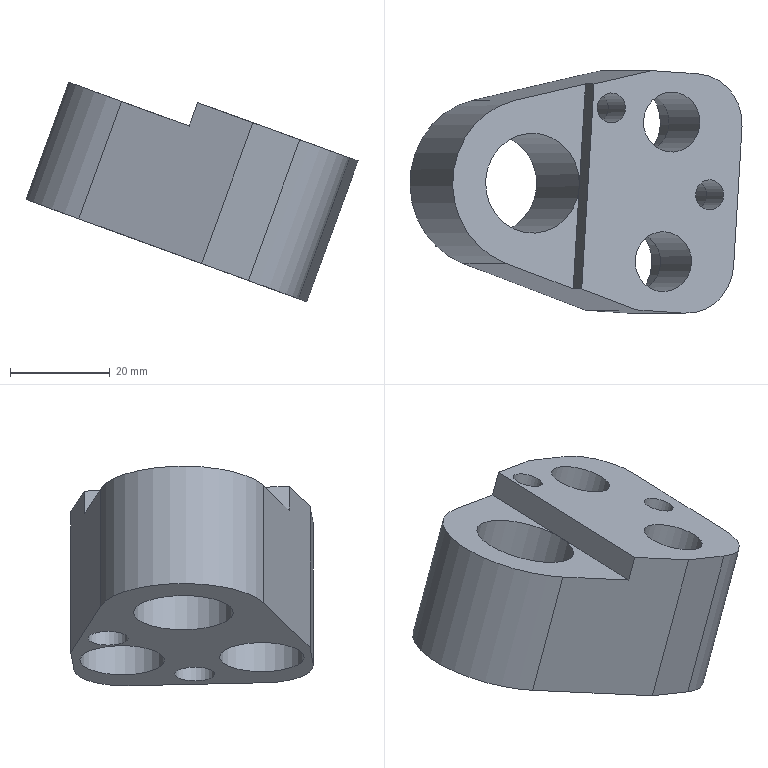Part | NX | features solid 2 | 1 solid | 25 faces | box 66.483 x 48.562 x 43.955 mm | volume 44567 mm3 | plane 13 | cylinder 12 | commonest cylinder face diameters 20 x3 6 x2 8 x2 12 x2 17 x2 34 x1
STEP:
#1=CARTESIAN_POINT('',(728.186,-470.964,2.295));
#2=VERTEX_POINT('',#1);
#3=CARTESIAN_POINT('',(731.937,-471.22,0.9298));
#4=DIRECTION('',(0.342,0.,0.9397));
#5=DIRECTION('',(-0.9378,0.06398,0.3413));
#6=AXIS2_PLACEMENT_3D('',#3,#4,#5);
#7=CIRCLE('',#6,4.);
#8=EDGE_CURVE('',#2,#2,#7,.F.);
#9=ORIENTED_EDGE('',*,*,#8,.F.);
#10=EDGE_LOOP('',(#9));
#11=FACE_BOUND('',#10,.T.);
#12=CARTESIAN_POINT('',(732.31,-457.217,0.7941));
#13=VERTEX_POINT('',#12);
#14=CARTESIAN_POINT('',(724.339,-456.673,3.695));
#15=DIRECTION('',(-0.342,0.,-0.9397));
#16=DIRECTION('',(0.9378,-0.06398,-0.3413));
#17=AXIS2_PLACEMENT_3D('',#14,#15,#16);
#18=CIRCLE('',#17,8.5);
#19=EDGE_CURVE('',#13,#13,#18,.T.);
#20=ORIENTED_EDGE('',*,*,#19,.F.);
#21=EDGE_LOOP('',(#20));
#22=FACE_BOUND('',#21,.T.);
#23=CARTESIAN_POINT('',(730.627,-485.159,1.407));
#24=VERTEX_POINT('',#23);
#25=CARTESIAN_POINT('',(722.656,-484.616,4.308));
#26=DIRECTION('',(-0.342,0.,-0.9397));
#27=DIRECTION('',(0.9378,-0.06398,-0.3413));
#28=AXIS2_PLACEMENT_3D('',#25,#26,#27);
#29=CIRCLE('',#28,8.5);
#30=EDGE_CURVE('',#24,#24,#29,.T.);
#31=ORIENTED_EDGE('',*,*,#30,.F.);
#32=EDGE_LOOP('',(#31));
#33=FACE_BOUND('',#32,.T.);
#34=CARTESIAN_POINT('',(688.8,-468.277,16.631));
#35=VERTEX_POINT('',#34);
#36=CARTESIAN_POINT('',(698.178,-468.917,13.217));
#37=DIRECTION('',(0.342,0.,0.9397));
#38=DIRECTION('',(-0.9378,0.06398,0.3413));
#39=AXIS2_PLACEMENT_3D('',#36,#37,#38);
#40=CIRCLE('',#39,10.);
#41=EDGE_CURVE('',#35,#35,#40,.T.);
#42=ORIENTED_EDGE('',*,*,#41,.T.);
#43=EDGE_LOOP('',(#42));
#44=FACE_BOUND('',#43,.T.);
#45=CARTESIAN_POINT('',(692.798,-484.924,15.176));
#46=VERTEX_POINT('',#45);
#47=CARTESIAN_POINT('',(717.366,-494.275,6.234));
#48=VERTEX_POINT('',#47);
#49=CARTESIAN_POINT('',(692.798,-484.924,15.176));
#50=DIRECTION('',(0.8848,-0.3368,-0.322));
#51=VECTOR('',#50,1000.);
#52=LINE('',#49,#51);
#53=EDGE_CURVE('',#46,#48,#52,.T.);
#54=ORIENTED_EDGE('',*,*,#53,.F.);
#55=CARTESIAN_POINT('',(694.762,-452.31,14.46));
#56=VERTEX_POINT('',#55);
#57=CARTESIAN_POINT('',(698.178,-468.917,13.217));
#58=DIRECTION('',(-0.342,0.,-0.9397));
#59=DIRECTION('',(0.9378,-0.06398,-0.3413));
#60=AXIS2_PLACEMENT_3D('',#57,#58,#59);
#61=CIRCLE('',#60,17.);
#62=EDGE_CURVE('',#46,#56,#61,.T.);
#63=ORIENTED_EDGE('',*,*,#62,.T.);
#64=CARTESIAN_POINT('',(720.252,-446.373,5.183));
#65=VERTEX_POINT('',#64);
#66=CARTESIAN_POINT('',(694.762,-452.31,14.46));
#67=DIRECTION('',(0.918,0.2138,-0.3341));
#68=VECTOR('',#67,1000.);
#69=LINE('',#66,#68);
#70=EDGE_CURVE('',#56,#65,#69,.T.);
#71=ORIENTED_EDGE('',*,*,#70,.T.);
#72=CARTESIAN_POINT('',(729.629,-447.013,1.77));
#73=VERTEX_POINT('',#72);
#74=CARTESIAN_POINT('',(720.252,-446.373,5.183));
#75=DIRECTION('',(0.9378,-0.06398,-0.3413));
#76=VECTOR('',#75,1000.);
#77=LINE('',#74,#76);
#78=EDGE_CURVE('',#65,#73,#77,.T.);
#79=ORIENTED_EDGE('',*,*,#78,.T.);
#80=CARTESIAN_POINT('',(738.406,-457.633,-1.424));
#81=VERTEX_POINT('',#80);
#82=CARTESIAN_POINT('',(729.028,-456.993,1.989));
#83=DIRECTION('',(-0.342,0.,-0.9397));
#84=DIRECTION('',(0.9378,-0.06398,-0.3413));
#85=AXIS2_PLACEMENT_3D('',#82,#83,#84);
#86=CIRCLE('',#85,10.);
#87=EDGE_CURVE('',#73,#81,#86,.T.);
#88=ORIENTED_EDGE('',*,*,#87,.T.);
#89=CARTESIAN_POINT('',(736.722,-485.575,-0.8117));
#90=VERTEX_POINT('',#89);
#91=CARTESIAN_POINT('',(736.722,-485.575,-0.8117));
#92=DIRECTION('',(0.06013,0.998,-0.02188));
#93=VECTOR('',#92,1000.);
#94=LINE('',#91,#93);
#95=EDGE_CURVE('',#90,#81,#94,.T.);
#96=ORIENTED_EDGE('',*,*,#95,.F.);
#97=CARTESIAN_POINT('',(726.743,-494.915,2.82));
#98=VERTEX_POINT('',#97);
#99=CARTESIAN_POINT('',(727.344,-484.935,2.601));
#100=DIRECTION('',(-0.342,0.,-0.9397));
#101=DIRECTION('',(0.9378,-0.06398,-0.3413));
#102=AXIS2_PLACEMENT_3D('',#99,#100,#101);
#103=CIRCLE('',#102,10.);
#104=EDGE_CURVE('',#90,#98,#103,.T.);
#105=ORIENTED_EDGE('',*,*,#104,.T.);
#106=CARTESIAN_POINT('',(717.366,-494.275,6.234));
#107=DIRECTION('',(0.9378,-0.06398,-0.3413));
#108=VECTOR('',#107,1000.);
#109=LINE('',#106,#108);
#110=EDGE_CURVE('',#48,#98,#109,.T.);
#111=ORIENTED_EDGE('',*,*,#110,.F.);
#112=EDGE_LOOP('',(#54,#63,#71,#79,#88,#96,#105,#111));
#113=FACE_BOUND('',#112,.T.);
#114=CARTESIAN_POINT('',(708.517,-453.589,9.454));
#115=VERTEX_POINT('',#114);
#116=CARTESIAN_POINT('',(712.268,-453.845,8.089));
#117=DIRECTION('',(0.342,0.,0.9397));
#118=DIRECTION('',(-0.9378,0.06398,0.3413));
#119=AXIS2_PLACEMENT_3D('',#116,#117,#118);
#120=CIRCLE('',#119,4.);
#121=EDGE_CURVE('',#115,#115,#120,.F.);
#122=ORIENTED_EDGE('',*,*,#121,.F.);
#123=EDGE_LOOP('',(#122));
#124=FACE_BOUND('',#123,.T.);
#125=CARTESIAN_POINT('',(727.344,-484.935,2.601));
#126=DIRECTION('',(-0.342,0.,-0.9397));
#127=DIRECTION('',(0.9378,-0.06398,-0.3413));
#128=AXIS2_PLACEMENT_3D('',#125,#126,#127);
#129=PLANE('',#128);
#130=ADVANCED_FACE('',(#11,#22,#33,#44,#113,#124),#129,.T.);
#131=CARTESIAN_POINT('',(745.011,-471.412,28.097));
#132=VERTEX_POINT('',#131);
#133=CARTESIAN_POINT('',(742.198,-471.22,29.121));
#134=DIRECTION('',(-0.342,0.,-0.9397));
#135=DIRECTION('',(0.9378,-0.06398,-0.3413));
#136=AXIS2_PLACEMENT_3D('',#133,#134,#135);
#137=CIRCLE('',#136,3.);
#138=EDGE_CURVE('',#132,#132,#137,.T.);
#139=ORIENTED_EDGE('',*,*,#138,.F.);
#140=EDGE_LOOP('',(#139));
#141=FACE_BOUND('',#140,.T.);
#142=CARTESIAN_POINT('',(741.591,-471.412,18.7));
#143=VERTEX_POINT('',#142);
#144=CARTESIAN_POINT('',(738.778,-471.22,19.724));
#145=DIRECTION('',(-0.342,0.,-0.9397));
#146=DIRECTION('',(0.9378,-0.06398,-0.3413));
#147=AXIS2_PLACEMENT_3D('',#144,#145,#146);
#148=CIRCLE('',#147,3.);
#149=EDGE_CURVE('',#143,#143,#148,.T.);
#150=ORIENTED_EDGE('',*,*,#149,.T.);
#151=EDGE_LOOP('',(#150));
#152=FACE_BOUND('',#151,.T.);
#153=CARTESIAN_POINT('',(731.937,-471.22,0.9298));
#154=DIRECTION('',(0.342,0.,0.9397));
#155=DIRECTION('',(-0.9378,0.06398,0.3413));
#156=AXIS2_PLACEMENT_3D('',#153,#154,#155);
#157=CYLINDRICAL_SURFACE('',#156,3.);
#158=ADVANCED_FACE('',(#141,#152),#157,.F.);
#159=CARTESIAN_POINT('',(740.226,-457.057,29.838));
#160=VERTEX_POINT('',#159);
#161=CARTESIAN_POINT('',(734.6,-456.673,31.886));
#162=DIRECTION('',(-0.342,0.,-0.9397));
#163=DIRECTION('',(0.9378,-0.06398,-0.3413));
#164=AXIS2_PLACEMENT_3D('',#161,#162,#163);
#165=CIRCLE('',#164,6.);
#166=EDGE_CURVE('',#160,#160,#165,.T.);
#167=ORIENTED_EDGE('',*,*,#166,.F.);
#168=EDGE_LOOP('',(#167));
#169=FACE_BOUND('',#168,.T.);
#170=CARTESIAN_POINT('',(734.07,-457.057,12.924));
#171=VERTEX_POINT('',#170);
#172=CARTESIAN_POINT('',(728.443,-456.673,14.972));
#173=DIRECTION('',(-0.342,0.,-0.9397));
#174=DIRECTION('',(0.9378,-0.06398,-0.3413));
#175=AXIS2_PLACEMENT_3D('',#172,#173,#174);
#176=CIRCLE('',#175,6.);
#177=EDGE_CURVE('',#171,#171,#176,.T.);
#178=ORIENTED_EDGE('',*,*,#177,.T.);
#179=EDGE_LOOP('',(#178));
#180=FACE_BOUND('',#179,.T.);
#181=CARTESIAN_POINT('',(724.339,-456.673,3.695));
#182=DIRECTION('',(0.342,0.,0.9397));
#183=DIRECTION('',(-0.9378,0.06398,0.3413));
#184=AXIS2_PLACEMENT_3D('',#181,#182,#183);
#185=CYLINDRICAL_SURFACE('',#184,6.);
#186=ADVANCED_FACE('',(#169,#180),#185,.F.);
#187=CARTESIAN_POINT('',(738.543,-484.999,30.451));
#188=VERTEX_POINT('',#187);
#189=CARTESIAN_POINT('',(732.916,-484.616,32.499));
#190=DIRECTION('',(-0.342,0.,-0.9397));
#191=DIRECTION('',(0.9378,-0.06398,-0.3413));
#192=AXIS2_PLACEMENT_3D('',#189,#190,#191);
#193=CIRCLE('',#192,6.);
#194=EDGE_CURVE('',#188,#188,#193,.T.);
#195=ORIENTED_EDGE('',*,*,#194,.F.);
#196=EDGE_LOOP('',(#195));
#197=FACE_BOUND('',#196,.T.);
#198=CARTESIAN_POINT('',(732.386,-484.999,13.536));
#199=VERTEX_POINT('',#198);
#200=CARTESIAN_POINT('',(726.76,-484.616,15.584));
#201=DIRECTION('',(-0.342,0.,-0.9397));
#202=DIRECTION('',(0.9378,-0.06398,-0.3413));
#203=AXIS2_PLACEMENT_3D('',#200,#201,#202);
#204=CIRCLE('',#203,6.);
#205=EDGE_CURVE('',#199,#199,#204,.T.);
#206=ORIENTED_EDGE('',*,*,#205,.T.);
#207=EDGE_LOOP('',(#206));
#208=FACE_BOUND('',#207,.T.);
#209=CARTESIAN_POINT('',(722.656,-484.616,4.308));
#210=DIRECTION('',(0.342,0.,0.9397));
#211=DIRECTION('',(-0.9378,0.06398,0.3413));
#212=AXIS2_PLACEMENT_3D('',#209,#210,#211);
#213=CYLINDRICAL_SURFACE('',#212,6.);
#214=ADVANCED_FACE('',(#197,#208),#213,.F.);
#215=CARTESIAN_POINT('',(725.342,-454.037,35.256));
#216=VERTEX_POINT('',#215);
#217=CARTESIAN_POINT('',(722.529,-453.845,36.279));
#218=DIRECTION('',(-0.342,0.,-0.9397));
#219=DIRECTION('',(0.9378,-0.06398,-0.3413));
#220=AXIS2_PLACEMENT_3D('',#217,#218,#219);
#221=CIRCLE('',#220,3.);
#222=EDGE_CURVE('',#216,#216,#221,.T.);
#223=ORIENTED_EDGE('',*,*,#222,.T.);
#224=EDGE_LOOP('',(#223));
#225=FACE_BOUND('',#224,.T.);
#226=ORIENTED_EDGE('',*,*,#166,.T.);
#227=EDGE_LOOP('',(#226));
#228=FACE_BOUND('',#227,.T.);
#229=CARTESIAN_POINT('',(719.052,-449.042,37.545));
#230=VERTEX_POINT('',#229);
#231=CARTESIAN_POINT('',(730.512,-446.373,33.374));
#232=VERTEX_POINT('',#231);
#233=CARTESIAN_POINT('',(705.023,-452.31,42.651));
#234=DIRECTION('',(0.918,0.2138,-0.3341));
#235=VECTOR('',#234,1000.);
#236=LINE('',#233,#235);
#237=EDGE_CURVE('',#230,#232,#236,.T.);
#238=ORIENTED_EDGE('',*,*,#237,.F.);
#239=CARTESIAN_POINT('',(716.58,-490.07,38.445));
#240=VERTEX_POINT('',#239);
#241=CARTESIAN_POINT('',(716.58,-490.07,38.445));
#242=DIRECTION('',(0.06013,0.998,-0.02188));
#243=VECTOR('',#242,1000.);
#244=LINE('',#241,#243);
#245=EDGE_CURVE('',#240,#230,#244,.T.);
#246=ORIENTED_EDGE('',*,*,#245,.F.);
#247=CARTESIAN_POINT('',(727.626,-494.275,34.424));
#248=VERTEX_POINT('',#247);
#249=CARTESIAN_POINT('',(703.058,-484.924,43.366));
#250=DIRECTION('',(0.8848,-0.3368,-0.322));
#251=VECTOR('',#250,1000.);
#252=LINE('',#249,#251);
#253=EDGE_CURVE('',#240,#248,#252,.T.);
#254=ORIENTED_EDGE('',*,*,#253,.T.);
#255=CARTESIAN_POINT('',(737.004,-494.915,31.011));
#256=VERTEX_POINT('',#255);
#257=CARTESIAN_POINT('',(727.626,-494.275,34.424));
#258=DIRECTION('',(0.9378,-0.06398,-0.3413));
#259=VECTOR('',#258,1000.);
#260=LINE('',#257,#259);
#261=EDGE_CURVE('',#248,#256,#260,.T.);
#262=ORIENTED_EDGE('',*,*,#261,.T.);
#263=CARTESIAN_POINT('',(746.983,-485.575,27.379));
#264=VERTEX_POINT('',#263);
#265=CARTESIAN_POINT('',(737.605,-484.935,30.792));
#266=DIRECTION('',(-0.342,0.,-0.9397));
#267=DIRECTION('',(0.9378,-0.06398,-0.3413));
#268=AXIS2_PLACEMENT_3D('',#265,#266,#267);
#269=CIRCLE('',#268,10.);
#270=EDGE_CURVE('',#264,#256,#269,.T.);
#271=ORIENTED_EDGE('',*,*,#270,.F.);
#272=CARTESIAN_POINT('',(748.666,-457.633,26.766));
#273=VERTEX_POINT('',#272);
#274=CARTESIAN_POINT('',(746.983,-485.575,27.379));
#275=DIRECTION('',(0.06013,0.998,-0.02188));
#276=VECTOR('',#275,1000.);
#277=LINE('',#274,#276);
#278=EDGE_CURVE('',#264,#273,#277,.T.);
#279=ORIENTED_EDGE('',*,*,#278,.T.);
#280=CARTESIAN_POINT('',(739.89,-447.013,29.961));
#281=VERTEX_POINT('',#280);
#282=CARTESIAN_POINT('',(739.289,-456.993,30.18));
#283=DIRECTION('',(-0.342,0.,-0.9397));
#284=DIRECTION('',(0.9378,-0.06398,-0.3413));
#285=AXIS2_PLACEMENT_3D('',#282,#283,#284);
#286=CIRCLE('',#285,10.);
#287=EDGE_CURVE('',#281,#273,#286,.T.);
#288=ORIENTED_EDGE('',*,*,#287,.F.);
#289=CARTESIAN_POINT('',(730.512,-446.373,33.374));
#290=DIRECTION('',(0.9378,-0.06398,-0.3413));
#291=VECTOR('',#290,1000.);
#292=LINE('',#289,#291);
#293=EDGE_CURVE('',#232,#281,#292,.T.);
#294=ORIENTED_EDGE('',*,*,#293,.F.);
#295=EDGE_LOOP('',(#238,#246,#254,#262,#271,#279,#288,#294));
#296=FACE_BOUND('',#295,.T.);
#297=ORIENTED_EDGE('',*,*,#194,.T.);
#298=EDGE_LOOP('',(#297));
#299=FACE_BOUND('',#298,.T.);
#300=ORIENTED_EDGE('',*,*,#138,.T.);
#301=EDGE_LOOP('',(#300));
#302=FACE_BOUND('',#301,.T.);
#303=CARTESIAN_POINT('',(737.605,-484.935,30.792));
#304=DIRECTION('',(-0.342,0.,-0.9397));
#305=DIRECTION('',(0.9378,-0.06398,-0.3413));
#306=AXIS2_PLACEMENT_3D('',#303,#304,#305);
#307=PLANE('',#306);
#308=ADVANCED_FACE('',(#225,#228,#296,#299,#302),#307,.F.);
#309=CARTESIAN_POINT('',(714.87,-490.07,33.746));
#310=VERTEX_POINT('',#309);
#311=CARTESIAN_POINT('',(714.87,-490.07,33.746));
#312=DIRECTION('',(0.342,0.,0.9397));
#313=VECTOR('',#312,1000.);
#314=LINE('',#311,#313);
#315=EDGE_CURVE('',#310,#240,#314,.T.);
#316=ORIENTED_EDGE('',*,*,#315,.F.);
#317=CARTESIAN_POINT('',(701.348,-484.924,38.668));
#318=VERTEX_POINT('',#317);
#319=CARTESIAN_POINT('',(714.87,-490.07,33.746));
#320=DIRECTION('',(-0.8848,0.3368,0.322));
#321=VECTOR('',#320,1000.);
#322=LINE('',#319,#321);
#323=EDGE_CURVE('',#310,#318,#322,.T.);
#324=ORIENTED_EDGE('',*,*,#323,.T.);
#325=CARTESIAN_POINT('',(692.798,-484.924,15.176));
#326=DIRECTION('',(0.342,0.,0.9397));
#327=VECTOR('',#326,1000.);
#328=LINE('',#325,#327);
#329=EDGE_CURVE('',#46,#318,#328,.T.);
#330=ORIENTED_EDGE('',*,*,#329,.F.);
#331=ORIENTED_EDGE('',*,*,#53,.T.);
#332=CARTESIAN_POINT('',(717.366,-494.275,6.234));
#333=DIRECTION('',(0.342,0.,0.9397));
#334=VECTOR('',#333,1000.);
#335=LINE('',#332,#334);
#336=EDGE_CURVE('',#48,#248,#335,.T.);
#337=ORIENTED_EDGE('',*,*,#336,.T.);
#338=ORIENTED_EDGE('',*,*,#253,.F.);
#339=EDGE_LOOP('',(#316,#324,#330,#331,#337,#338));
#340=FACE_BOUND('',#339,.T.);
#341=CARTESIAN_POINT('',(692.798,-484.924,15.176));
#342=DIRECTION('',(-0.3165,-0.9416,0.1152));
#343=DIRECTION('',(0.8848,-0.3368,-0.322));
#344=AXIS2_PLACEMENT_3D('',#341,#342,#343);
#345=PLANE('',#344);
#346=ADVANCED_FACE('',(#340),#345,.T.);
#347=ORIENTED_EDGE('',*,*,#261,.F.);
#348=ORIENTED_EDGE('',*,*,#336,.F.);
#349=ORIENTED_EDGE('',*,*,#110,.T.);
#350=CARTESIAN_POINT('',(726.743,-494.915,2.82));
#351=DIRECTION('',(0.342,0.,0.9397));
#352=VECTOR('',#351,1000.);
#353=LINE('',#350,#352);
#354=EDGE_CURVE('',#98,#256,#353,.T.);
#355=ORIENTED_EDGE('',*,*,#354,.T.);
#356=EDGE_LOOP('',(#347,#348,#349,#355));
#357=FACE_BOUND('',#356,.T.);
#358=CARTESIAN_POINT('',(717.366,-494.275,6.234));
#359=DIRECTION('',(-0.06013,-0.998,0.02188));
#360=DIRECTION('',(0.9378,-0.06398,-0.3413));
#361=AXIS2_PLACEMENT_3D('',#358,#359,#360);
#362=PLANE('',#361);
#363=ADVANCED_FACE('',(#357),#362,.T.);
#364=ORIENTED_EDGE('',*,*,#270,.T.);
#365=ORIENTED_EDGE('',*,*,#354,.F.);
#366=ORIENTED_EDGE('',*,*,#104,.F.);
#367=CARTESIAN_POINT('',(736.722,-485.575,-0.8117));
#368=DIRECTION('',(0.342,0.,0.9397));
#369=VECTOR('',#368,1000.);
#370=LINE('',#367,#369);
#371=EDGE_CURVE('',#90,#264,#370,.T.);
#372=ORIENTED_EDGE('',*,*,#371,.T.);
#373=EDGE_LOOP('',(#364,#365,#366,#372));
#374=FACE_BOUND('',#373,.T.);
#375=CARTESIAN_POINT('',(727.344,-484.935,2.601));
#376=DIRECTION('',(0.342,0.,0.9397));
#377=DIRECTION('',(-0.9378,0.06398,0.3413));
#378=AXIS2_PLACEMENT_3D('',#375,#376,#377);
#379=CYLINDRICAL_SURFACE('',#378,10.);
#380=ADVANCED_FACE('',(#374),#379,.T.);
#381=ORIENTED_EDGE('',*,*,#278,.F.);
#382=ORIENTED_EDGE('',*,*,#371,.F.);
#383=ORIENTED_EDGE('',*,*,#95,.T.);
#384=CARTESIAN_POINT('',(738.406,-457.633,-1.424));
#385=DIRECTION('',(0.342,0.,0.9397));
#386=VECTOR('',#385,1000.);
#387=LINE('',#384,#386);
#388=EDGE_CURVE('',#81,#273,#387,.T.);
#389=ORIENTED_EDGE('',*,*,#388,.T.);
#390=EDGE_LOOP('',(#381,#382,#383,#389));
#391=FACE_BOUND('',#390,.T.);
#392=CARTESIAN_POINT('',(736.722,-485.575,-0.8117));
#393=DIRECTION('',(0.9378,-0.06398,-0.3413));
#394=DIRECTION('',(0.06013,0.998,-0.02188));
#395=AXIS2_PLACEMENT_3D('',#392,#393,#394);
#396=PLANE('',#395);
#397=ADVANCED_FACE('',(#391),#396,.T.);
#398=ORIENTED_EDGE('',*,*,#287,.T.);
#399=ORIENTED_EDGE('',*,*,#388,.F.);
#400=ORIENTED_EDGE('',*,*,#87,.F.);
#401=CARTESIAN_POINT('',(729.629,-447.013,1.77));
#402=DIRECTION('',(0.342,0.,0.9397));
#403=VECTOR('',#402,1000.);
#404=LINE('',#401,#403);
#405=EDGE_CURVE('',#73,#281,#404,.T.);
#406=ORIENTED_EDGE('',*,*,#405,.T.);
#407=EDGE_LOOP('',(#398,#399,#400,#406));
#408=FACE_BOUND('',#407,.T.);
#409=CARTESIAN_POINT('',(729.028,-456.993,1.989));
#410=DIRECTION('',(0.342,0.,0.9397));
#411=DIRECTION('',(-0.9378,0.06398,0.3413));
#412=AXIS2_PLACEMENT_3D('',#409,#410,#411);
#413=CYLINDRICAL_SURFACE('',#412,10.);
#414=ADVANCED_FACE('',(#408),#413,.T.);
#415=ORIENTED_EDGE('',*,*,#293,.T.);
#416=ORIENTED_EDGE('',*,*,#405,.F.);
#417=ORIENTED_EDGE('',*,*,#78,.F.);
#418=CARTESIAN_POINT('',(720.252,-446.373,5.183));
#419=DIRECTION('',(0.342,0.,0.9397));
#420=VECTOR('',#419,1000.);
#421=LINE('',#418,#420);
#422=EDGE_CURVE('',#65,#232,#421,.T.);
#423=ORIENTED_EDGE('',*,*,#422,.T.);
#424=EDGE_LOOP('',(#415,#416,#417,#423));
#425=FACE_BOUND('',#424,.T.);
#426=CARTESIAN_POINT('',(720.252,-446.373,5.183));
#427=DIRECTION('',(-0.06013,-0.998,0.02188));
#428=DIRECTION('',(0.342,0.,0.9397));
#429=AXIS2_PLACEMENT_3D('',#426,#427,#428);
#430=PLANE('',#429);
#431=ADVANCED_FACE('',(#425),#430,.F.);
#432=CARTESIAN_POINT('',(717.342,-449.042,32.847));
#433=VERTEX_POINT('',#432);
#434=CARTESIAN_POINT('',(703.313,-452.31,37.953));
#435=VERTEX_POINT('',#434);
#436=CARTESIAN_POINT('',(717.342,-449.042,32.847));
#437=DIRECTION('',(-0.918,-0.2138,0.3341));
#438=VECTOR('',#437,1000.);
#439=LINE('',#436,#438);
#440=EDGE_CURVE('',#433,#435,#439,.T.);
#441=ORIENTED_EDGE('',*,*,#440,.F.);
#442=CARTESIAN_POINT('',(717.342,-449.042,32.847));
#443=DIRECTION('',(0.342,0.,0.9397));
#444=VECTOR('',#443,1000.);
#445=LINE('',#442,#444);
#446=EDGE_CURVE('',#433,#230,#445,.T.);
#447=ORIENTED_EDGE('',*,*,#446,.T.);
#448=ORIENTED_EDGE('',*,*,#237,.T.);
#449=ORIENTED_EDGE('',*,*,#422,.F.);
#450=ORIENTED_EDGE('',*,*,#70,.F.);
#451=CARTESIAN_POINT('',(694.762,-452.31,14.46));
#452=DIRECTION('',(0.342,0.,0.9397));
#453=VECTOR('',#452,1000.);
#454=LINE('',#451,#453);
#455=EDGE_CURVE('',#56,#435,#454,.T.);
#456=ORIENTED_EDGE('',*,*,#455,.T.);
#457=EDGE_LOOP('',(#441,#447,#448,#449,#450,#456));
#458=FACE_BOUND('',#457,.T.);
#459=CARTESIAN_POINT('',(694.762,-452.31,14.46));
#460=DIRECTION('',(0.2009,-0.9769,-0.07312));
#461=DIRECTION('',(0.918,0.2138,-0.3341));
#462=AXIS2_PLACEMENT_3D('',#459,#460,#461);
#463=PLANE('',#462);
#464=ADVANCED_FACE('',(#458),#463,.F.);
#465=ORIENTED_EDGE('',*,*,#329,.T.);
#466=CARTESIAN_POINT('',(706.728,-468.917,36.71));
#467=DIRECTION('',(-0.342,0.,-0.9397));
#468=DIRECTION('',(0.9378,-0.06398,-0.3413));
#469=AXIS2_PLACEMENT_3D('',#466,#467,#468);
#470=CIRCLE('',#469,17.);
#471=EDGE_CURVE('',#318,#435,#470,.T.);
#472=ORIENTED_EDGE('',*,*,#471,.T.);
#473=ORIENTED_EDGE('',*,*,#455,.F.);
#474=ORIENTED_EDGE('',*,*,#62,.F.);
#475=EDGE_LOOP('',(#465,#472,#473,#474));
#476=FACE_BOUND('',#475,.T.);
#477=CARTESIAN_POINT('',(698.178,-468.917,13.217));
#478=DIRECTION('',(0.342,0.,0.9397));
#479=DIRECTION('',(-0.9378,0.06398,0.3413));
#480=AXIS2_PLACEMENT_3D('',#477,#478,#479);
#481=CYLINDRICAL_SURFACE('',#480,17.);
#482=ADVANCED_FACE('',(#476),#481,.T.);
#483=CARTESIAN_POINT('',(716.106,-469.556,33.296));
#484=VERTEX_POINT('',#483);
#485=CARTESIAN_POINT('',(706.728,-468.917,36.71));
#486=DIRECTION('',(-0.342,0.,-0.9397));
#487=DIRECTION('',(0.9378,-0.06398,-0.3413));
#488=AXIS2_PLACEMENT_3D('',#485,#486,#487);
#489=CIRCLE('',#488,10.);
#490=EDGE_CURVE('',#484,#484,#489,.F.);
#491=ORIENTED_EDGE('',*,*,#490,.T.);
#492=EDGE_LOOP('',(#491));
#493=FACE_BOUND('',#492,.T.);
#494=ORIENTED_EDGE('',*,*,#41,.F.);
#495=EDGE_LOOP('',(#494));
#496=FACE_BOUND('',#495,.T.);
#497=CARTESIAN_POINT('',(698.178,-468.917,13.217));
#498=DIRECTION('',(0.342,0.,0.9397));
#499=DIRECTION('',(-0.9378,0.06398,0.3413));
#500=AXIS2_PLACEMENT_3D('',#497,#498,#499);
#501=CYLINDRICAL_SURFACE('',#500,10.);
#502=ADVANCED_FACE('',(#493,#496),#501,.F.);
#503=ORIENTED_EDGE('',*,*,#245,.T.);
#504=ORIENTED_EDGE('',*,*,#446,.F.);
#505=CARTESIAN_POINT('',(714.87,-490.07,33.746));
#506=DIRECTION('',(0.06013,0.998,-0.02188));
#507=VECTOR('',#506,1000.);
#508=LINE('',#505,#507);
#509=EDGE_CURVE('',#484,#433,#508,.T.);
#510=ORIENTED_EDGE('',*,*,#509,.F.);
#511=CARTESIAN_POINT('',(714.87,-490.07,33.746));
#512=DIRECTION('',(0.06013,0.998,-0.02188));
#513=VECTOR('',#512,1000.);
#514=LINE('',#511,#513);
#515=EDGE_CURVE('',#310,#484,#514,.T.);
#516=ORIENTED_EDGE('',*,*,#515,.F.);
#517=ORIENTED_EDGE('',*,*,#315,.T.);
#518=EDGE_LOOP('',(#503,#504,#510,#516,#517));
#519=FACE_BOUND('',#518,.T.);
#520=CARTESIAN_POINT('',(714.87,-490.07,33.746));
#521=DIRECTION('',(0.9378,-0.06398,-0.3413));
#522=DIRECTION('',(0.06013,0.998,-0.02188));
#523=AXIS2_PLACEMENT_3D('',#520,#521,#522);
#524=PLANE('',#523);
#525=ADVANCED_FACE('',(#519),#524,.F.);
#526=ORIENTED_EDGE('',*,*,#509,.T.);
#527=ORIENTED_EDGE('',*,*,#440,.T.);
#528=ORIENTED_EDGE('',*,*,#471,.F.);
#529=ORIENTED_EDGE('',*,*,#323,.F.);
#530=ORIENTED_EDGE('',*,*,#515,.T.);
#531=ORIENTED_EDGE('',*,*,#490,.F.);
#532=EDGE_LOOP('',(#526,#527,#528,#529,#530,#531));
#533=FACE_BOUND('',#532,.T.);
#534=CARTESIAN_POINT('',(706.728,-468.917,36.71));
#535=DIRECTION('',(-0.342,0.,-0.9397));
#536=DIRECTION('',(0.9378,-0.06398,-0.3413));
#537=AXIS2_PLACEMENT_3D('',#534,#535,#536);
#538=PLANE('',#537);
#539=ADVANCED_FACE('',(#533),#538,.F.);
#540=CARTESIAN_POINT('',(721.922,-454.037,25.859));
#541=VERTEX_POINT('',#540);
#542=CARTESIAN_POINT('',(719.109,-453.845,26.883));
#543=DIRECTION('',(-0.342,0.,-0.9397));
#544=DIRECTION('',(0.9378,-0.06398,-0.3413));
#545=AXIS2_PLACEMENT_3D('',#542,#543,#544);
#546=CIRCLE('',#545,3.);
#547=EDGE_CURVE('',#541,#541,#546,.T.);
#548=ORIENTED_EDGE('',*,*,#547,.T.);
#549=EDGE_LOOP('',(#548));
#550=FACE_BOUND('',#549,.T.);
#551=ORIENTED_EDGE('',*,*,#222,.F.);
#552=EDGE_LOOP('',(#551));
#553=FACE_BOUND('',#552,.T.);
#554=CARTESIAN_POINT('',(712.268,-453.845,8.089));
#555=DIRECTION('',(0.342,0.,0.9397));
#556=DIRECTION('',(-0.9378,0.06398,0.3413));
#557=AXIS2_PLACEMENT_3D('',#554,#555,#556);
#558=CYLINDRICAL_SURFACE('',#557,3.);
#559=ADVANCED_FACE('',(#550,#553),#558,.F.);
#560=CARTESIAN_POINT('',(734.731,-485.159,12.683));
#561=VERTEX_POINT('',#560);
#562=CARTESIAN_POINT('',(726.76,-484.616,15.584));
#563=DIRECTION('',(-0.342,0.,-0.9397));
#564=DIRECTION('',(0.9378,-0.06398,-0.3413));
#565=AXIS2_PLACEMENT_3D('',#562,#563,#564);
#566=CIRCLE('',#565,8.5);
#567=EDGE_CURVE('',#561,#561,#566,.T.);
#568=ORIENTED_EDGE('',*,*,#567,.F.);
#569=EDGE_LOOP('',(#568));
#570=FACE_BOUND('',#569,.T.);
#571=ORIENTED_EDGE('',*,*,#30,.T.);
#572=EDGE_LOOP('',(#571));
#573=FACE_BOUND('',#572,.T.);
#574=CARTESIAN_POINT('',(726.76,-484.616,15.584));
#575=DIRECTION('',(-0.342,0.,-0.9397));
#576=DIRECTION('',(0.9378,-0.06398,-0.3413));
#577=AXIS2_PLACEMENT_3D('',#574,#575,#576);
#578=CYLINDRICAL_SURFACE('',#577,8.5);
#579=ADVANCED_FACE('',(#570,#573),#578,.F.);
#580=ORIENTED_EDGE('',*,*,#205,.F.);
#581=EDGE_LOOP('',(#580));
#582=FACE_BOUND('',#581,.T.);
#583=ORIENTED_EDGE('',*,*,#567,.T.);
#584=EDGE_LOOP('',(#583));
#585=FACE_BOUND('',#584,.T.);
#586=CARTESIAN_POINT('',(726.76,-484.616,15.584));
#587=DIRECTION('',(-0.342,0.,-0.9397));
#588=DIRECTION('',(0.9378,-0.06398,-0.3413));
#589=AXIS2_PLACEMENT_3D('',#586,#587,#588);
#590=PLANE('',#589);
#591=ADVANCED_FACE('',(#582,#585),#590,.T.);
#592=CARTESIAN_POINT('',(736.414,-457.217,12.07));
#593=VERTEX_POINT('',#592);
#594=CARTESIAN_POINT('',(728.443,-456.673,14.972));
#595=DIRECTION('',(-0.342,0.,-0.9397));
#596=DIRECTION('',(0.9378,-0.06398,-0.3413));
#597=AXIS2_PLACEMENT_3D('',#594,#595,#596);
#598=CIRCLE('',#597,8.5);
#599=EDGE_CURVE('',#593,#593,#598,.T.);
#600=ORIENTED_EDGE('',*,*,#599,.F.);
#601=EDGE_LOOP('',(#600));
#602=FACE_BOUND('',#601,.T.);
#603=ORIENTED_EDGE('',*,*,#19,.T.);
#604=EDGE_LOOP('',(#603));
#605=FACE_BOUND('',#604,.T.);
#606=CARTESIAN_POINT('',(728.443,-456.673,14.972));
#607=DIRECTION('',(-0.342,0.,-0.9397));
#608=DIRECTION('',(0.9378,-0.06398,-0.3413));
#609=AXIS2_PLACEMENT_3D('',#606,#607,#608);
#610=CYLINDRICAL_SURFACE('',#609,8.5);
#611=ADVANCED_FACE('',(#602,#605),#610,.F.);
#612=ORIENTED_EDGE('',*,*,#177,.F.);
#613=EDGE_LOOP('',(#612));
#614=FACE_BOUND('',#613,.T.);
#615=ORIENTED_EDGE('',*,*,#599,.T.);
#616=EDGE_LOOP('',(#615));
#617=FACE_BOUND('',#616,.T.);
#618=CARTESIAN_POINT('',(728.443,-456.673,14.972));
#619=DIRECTION('',(-0.342,0.,-0.9397));
#620=DIRECTION('',(0.9378,-0.06398,-0.3413));
#621=AXIS2_PLACEMENT_3D('',#618,#619,#620);
#622=PLANE('',#621);
#623=ADVANCED_FACE('',(#614,#617),#622,.T.);
#624=ORIENTED_EDGE('',*,*,#149,.F.);
#625=EDGE_LOOP('',(#624));
#626=FACE_BOUND('',#625,.T.);
#627=CARTESIAN_POINT('',(735.027,-470.964,21.089));
#628=VERTEX_POINT('',#627);
#629=CARTESIAN_POINT('',(738.778,-471.22,19.724));
#630=DIRECTION('',(0.342,0.,0.9397));
#631=DIRECTION('',(-0.9378,0.06398,0.3413));
#632=AXIS2_PLACEMENT_3D('',#629,#630,#631);
#633=CIRCLE('',#632,4.);
#634=EDGE_CURVE('',#628,#628,#633,.F.);
#635=ORIENTED_EDGE('',*,*,#634,.T.);
#636=EDGE_LOOP('',(#635));
#637=FACE_BOUND('',#636,.T.);
#638=CARTESIAN_POINT('',(738.778,-471.22,19.724));
#639=DIRECTION('',(0.342,0.,0.9397));
#640=DIRECTION('',(-0.9378,0.06398,0.3413));
#641=AXIS2_PLACEMENT_3D('',#638,#639,#640);
#642=PLANE('',#641);
#643=ADVANCED_FACE('',(#626,#637),#642,.F.);
#644=ORIENTED_EDGE('',*,*,#634,.F.);
#645=EDGE_LOOP('',(#644));
#646=FACE_BOUND('',#645,.T.);
#647=ORIENTED_EDGE('',*,*,#8,.T.);
#648=EDGE_LOOP('',(#647));
#649=FACE_BOUND('',#648,.T.);
#650=CARTESIAN_POINT('',(731.937,-471.22,0.9298));
#651=DIRECTION('',(0.342,0.,0.9397));
#652=DIRECTION('',(-0.9378,0.06398,0.3413));
#653=AXIS2_PLACEMENT_3D('',#650,#651,#652);
#654=CYLINDRICAL_SURFACE('',#653,4.);
#655=ADVANCED_FACE('',(#646,#649),#654,.F.);
#656=ORIENTED_EDGE('',*,*,#547,.F.);
#657=EDGE_LOOP('',(#656));
#658=FACE_BOUND('',#657,.T.);
#659=CARTESIAN_POINT('',(715.358,-453.589,28.248));
#660=VERTEX_POINT('',#659);
#661=CARTESIAN_POINT('',(719.109,-453.845,26.883));
#662=DIRECTION('',(0.342,0.,0.9397));
#663=DIRECTION('',(-0.9378,0.06398,0.3413));
#664=AXIS2_PLACEMENT_3D('',#661,#662,#663);
#665=CIRCLE('',#664,4.);
#666=EDGE_CURVE('',#660,#660,#665,.F.);
#667=ORIENTED_EDGE('',*,*,#666,.T.);
#668=EDGE_LOOP('',(#667));
#669=FACE_BOUND('',#668,.T.);
#670=CARTESIAN_POINT('',(719.109,-453.845,26.883));
#671=DIRECTION('',(0.342,0.,0.9397));
#672=DIRECTION('',(-0.9378,0.06398,0.3413));
#673=AXIS2_PLACEMENT_3D('',#670,#671,#672);
#674=PLANE('',#673);
#675=ADVANCED_FACE('',(#658,#669),#674,.F.);
#676=ORIENTED_EDGE('',*,*,#666,.F.);
#677=EDGE_LOOP('',(#676));
#678=FACE_BOUND('',#677,.T.);
#679=ORIENTED_EDGE('',*,*,#121,.T.);
#680=EDGE_LOOP('',(#679));
#681=FACE_BOUND('',#680,.T.);
#682=CARTESIAN_POINT('',(712.268,-453.845,8.089));
#683=DIRECTION('',(0.342,0.,0.9397));
#684=DIRECTION('',(-0.9378,0.06398,0.3413));
#685=AXIS2_PLACEMENT_3D('',#682,#683,#684);
#686=CYLINDRICAL_SURFACE('',#685,4.);
#687=ADVANCED_FACE('',(#678,#681),#686,.F.);
#688=CLOSED_SHELL('',(#130,#158,#186,#214,#308,#346,#363,#380,#397,#414,#431,#464,#482,#502,#525,#539,#559,#579,#591,#611,#623,#643,#655,#675,#687));
#689=MANIFOLD_SOLID_BREP('',#688);
#690=(LENGTH_UNIT()NAMED_UNIT(*)SI_UNIT(.MILLI.,.METRE.));
#691=UNCERTAINTY_MEASURE_WITH_UNIT(LENGTH_MEASURE(0.00001),#690,'','');
#692=(NAMED_UNIT(*)PLANE_ANGLE_UNIT()SI_UNIT($,.RADIAN.));
#693=(NAMED_UNIT(*)SI_UNIT($,.STERADIAN.)SOLID_ANGLE_UNIT());
#694=(GEOMETRIC_REPRESENTATION_CONTEXT(3)GLOBAL_UNCERTAINTY_ASSIGNED_CONTEXT((#691))GLOBAL_UNIT_ASSIGNED_CONTEXT((#690,#692,#693))REPRESENTATION_CONTEXT('',''));
#695=ADVANCED_BREP_SHAPE_REPRESENTATION('',(#689),#694);